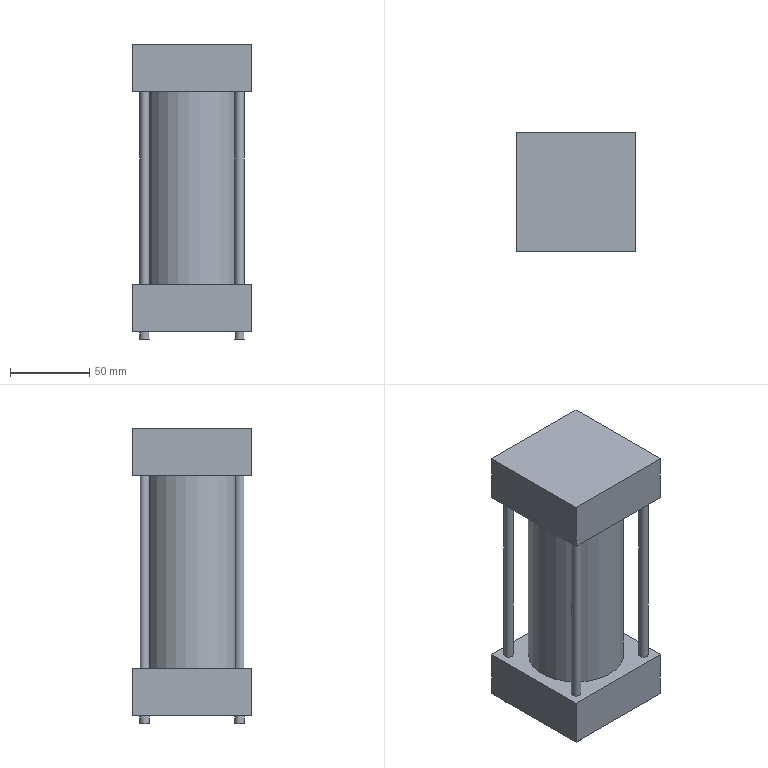Part | NX | features solid 2 | 1 solid | 29 faces | box 75 x 75 x 186 mm | volume 689867 mm3 | plane 16 | cylinder 13 | commonest cylinder face diameters 6 x8 60 x3 18 x2
STEP:
#1=CARTESIAN_POINT('',(168.,47.5,-150.));
#2=VERTEX_POINT('',#1);
#3=CARTESIAN_POINT('',(165.,47.5,-150.));
#4=DIRECTION('',(0.,0.,1.));
#5=DIRECTION('',(1.,0.,0.));
#6=AXIS2_PLACEMENT_3D('',#3,#4,#5);
#7=CIRCLE('',#6,3.);
#8=EDGE_CURVE('',#2,#2,#7,.F.);
#9=ORIENTED_EDGE('',*,*,#8,.F.);
#10=EDGE_LOOP('',(#9));
#11=FACE_BOUND('',#10,.T.);
#12=CARTESIAN_POINT('',(108.,47.5,-150.));
#13=VERTEX_POINT('',#12);
#14=CARTESIAN_POINT('',(105.,47.5,-150.));
#15=DIRECTION('',(0.,0.,1.));
#16=DIRECTION('',(1.,0.,0.));
#17=AXIS2_PLACEMENT_3D('',#14,#15,#16);
#18=CIRCLE('',#17,3.);
#19=EDGE_CURVE('',#13,#13,#18,.T.);
#20=ORIENTED_EDGE('',*,*,#19,.T.);
#21=EDGE_LOOP('',(#20));
#22=FACE_BOUND('',#21,.T.);
#23=CARTESIAN_POINT('',(97.5,115.,-150.));
#24=VERTEX_POINT('',#23);
#25=CARTESIAN_POINT('',(97.5,40.,-150.));
#26=VERTEX_POINT('',#25);
#27=CARTESIAN_POINT('',(97.5,112.5,-150.));
#28=DIRECTION('',(0.,-1.,0.));
#29=VECTOR('',#28,1000.);
#30=LINE('',#27,#29);
#31=EDGE_CURVE('',#24,#26,#30,.T.);
#32=ORIENTED_EDGE('',*,*,#31,.F.);
#33=CARTESIAN_POINT('',(172.5,115.,-150.));
#34=VERTEX_POINT('',#33);
#35=CARTESIAN_POINT('',(170.,115.,-150.));
#36=DIRECTION('',(-1.,0.,0.));
#37=VECTOR('',#36,1000.);
#38=LINE('',#35,#37);
#39=EDGE_CURVE('',#34,#24,#38,.T.);
#40=ORIENTED_EDGE('',*,*,#39,.F.);
#41=CARTESIAN_POINT('',(172.5,40.,-150.));
#42=VERTEX_POINT('',#41);
#43=CARTESIAN_POINT('',(172.5,42.5,-150.));
#44=DIRECTION('',(0.,1.,0.));
#45=VECTOR('',#44,1000.);
#46=LINE('',#43,#45);
#47=EDGE_CURVE('',#42,#34,#46,.T.);
#48=ORIENTED_EDGE('',*,*,#47,.F.);
#49=CARTESIAN_POINT('',(100.,40.,-150.));
#50=DIRECTION('',(1.,0.,0.));
#51=VECTOR('',#50,1000.);
#52=LINE('',#49,#51);
#53=EDGE_CURVE('',#26,#42,#52,.T.);
#54=ORIENTED_EDGE('',*,*,#53,.F.);
#55=EDGE_LOOP('',(#32,#40,#48,#54));
#56=FACE_BOUND('',#55,.T.);
#57=CARTESIAN_POINT('',(168.,107.5,-150.));
#58=VERTEX_POINT('',#57);
#59=CARTESIAN_POINT('',(165.,107.5,-150.));
#60=DIRECTION('',(0.,0.,1.));
#61=DIRECTION('',(1.,0.,0.));
#62=AXIS2_PLACEMENT_3D('',#59,#60,#61);
#63=CIRCLE('',#62,3.);
#64=EDGE_CURVE('',#58,#58,#63,.T.);
#65=ORIENTED_EDGE('',*,*,#64,.T.);
#66=EDGE_LOOP('',(#65));
#67=FACE_BOUND('',#66,.T.);
#68=CARTESIAN_POINT('',(108.,107.5,-150.));
#69=VERTEX_POINT('',#68);
#70=CARTESIAN_POINT('',(105.,107.5,-150.));
#71=DIRECTION('',(0.,0.,1.));
#72=DIRECTION('',(1.,0.,0.));
#73=AXIS2_PLACEMENT_3D('',#70,#71,#72);
#74=CIRCLE('',#73,3.);
#75=EDGE_CURVE('',#69,#69,#74,.F.);
#76=ORIENTED_EDGE('',*,*,#75,.F.);
#77=EDGE_LOOP('',(#76));
#78=FACE_BOUND('',#77,.T.);
#79=CARTESIAN_POINT('',(165.,77.5,-150.));
#80=VERTEX_POINT('',#79);
#81=CARTESIAN_POINT('',(135.,77.5,-150.));
#82=DIRECTION('',(0.,0.,1.));
#83=DIRECTION('',(1.,0.,0.));
#84=AXIS2_PLACEMENT_3D('',#81,#82,#83);
#85=CIRCLE('',#84,30.);
#86=EDGE_CURVE('',#80,#80,#85,.F.);
#87=ORIENTED_EDGE('',*,*,#86,.F.);
#88=EDGE_LOOP('',(#87));
#89=FACE_BOUND('',#88,.T.);
#90=CARTESIAN_POINT('',(100.,42.5,-150.));
#91=DIRECTION('',(0.,0.,-1.));
#92=DIRECTION('',(1.,0.,0.));
#93=AXIS2_PLACEMENT_3D('',#90,#91,#92);
#94=PLANE('',#93);
#95=ADVANCED_FACE('',(#11,#22,#56,#67,#78,#89),#94,.T.);
#96=CARTESIAN_POINT('',(108.,107.5,-271.));
#97=VERTEX_POINT('',#96);
#98=CARTESIAN_POINT('',(105.,107.5,-271.));
#99=DIRECTION('',(0.,0.,1.));
#100=DIRECTION('',(1.,0.,0.));
#101=AXIS2_PLACEMENT_3D('',#98,#99,#100);
#102=CIRCLE('',#101,3.);
#103=EDGE_CURVE('',#97,#97,#102,.T.);
#104=ORIENTED_EDGE('',*,*,#103,.F.);
#105=EDGE_LOOP('',(#104));
#106=FACE_BOUND('',#105,.T.);
#107=CARTESIAN_POINT('',(108.,47.5,-271.));
#108=VERTEX_POINT('',#107);
#109=CARTESIAN_POINT('',(105.,47.5,-271.));
#110=DIRECTION('',(0.,0.,1.));
#111=DIRECTION('',(1.,0.,0.));
#112=AXIS2_PLACEMENT_3D('',#109,#110,#111);
#113=CIRCLE('',#112,3.);
#114=EDGE_CURVE('',#108,#108,#113,.F.);
#115=ORIENTED_EDGE('',*,*,#114,.T.);
#116=EDGE_LOOP('',(#115));
#117=FACE_BOUND('',#116,.T.);
#118=CARTESIAN_POINT('',(172.5,40.,-271.));
#119=VERTEX_POINT('',#118);
#120=CARTESIAN_POINT('',(172.5,115.,-271.));
#121=VERTEX_POINT('',#120);
#122=CARTESIAN_POINT('',(172.5,42.5,-271.));
#123=DIRECTION('',(0.,1.,0.));
#124=VECTOR('',#123,1000.);
#125=LINE('',#122,#124);
#126=EDGE_CURVE('',#119,#121,#125,.T.);
#127=ORIENTED_EDGE('',*,*,#126,.T.);
#128=CARTESIAN_POINT('',(97.5,115.,-271.));
#129=VERTEX_POINT('',#128);
#130=CARTESIAN_POINT('',(170.,115.,-271.));
#131=DIRECTION('',(-1.,0.,0.));
#132=VECTOR('',#131,1000.);
#133=LINE('',#130,#132);
#134=EDGE_CURVE('',#121,#129,#133,.T.);
#135=ORIENTED_EDGE('',*,*,#134,.T.);
#136=CARTESIAN_POINT('',(97.5,40.,-271.));
#137=VERTEX_POINT('',#136);
#138=CARTESIAN_POINT('',(97.5,112.5,-271.));
#139=DIRECTION('',(0.,-1.,0.));
#140=VECTOR('',#139,1000.);
#141=LINE('',#138,#140);
#142=EDGE_CURVE('',#129,#137,#141,.T.);
#143=ORIENTED_EDGE('',*,*,#142,.T.);
#144=CARTESIAN_POINT('',(100.,40.,-271.));
#145=DIRECTION('',(1.,0.,0.));
#146=VECTOR('',#145,1000.);
#147=LINE('',#144,#146);
#148=EDGE_CURVE('',#137,#119,#147,.T.);
#149=ORIENTED_EDGE('',*,*,#148,.T.);
#150=EDGE_LOOP('',(#127,#135,#143,#149));
#151=FACE_BOUND('',#150,.T.);
#152=CARTESIAN_POINT('',(168.,47.5,-271.));
#153=VERTEX_POINT('',#152);
#154=CARTESIAN_POINT('',(165.,47.5,-271.));
#155=DIRECTION('',(0.,0.,1.));
#156=DIRECTION('',(1.,0.,0.));
#157=AXIS2_PLACEMENT_3D('',#154,#155,#156);
#158=CIRCLE('',#157,3.);
#159=EDGE_CURVE('',#153,#153,#158,.T.);
#160=ORIENTED_EDGE('',*,*,#159,.F.);
#161=EDGE_LOOP('',(#160));
#162=FACE_BOUND('',#161,.T.);
#163=CARTESIAN_POINT('',(168.,107.5,-271.));
#164=VERTEX_POINT('',#163);
#165=CARTESIAN_POINT('',(165.,107.5,-271.));
#166=DIRECTION('',(0.,0.,1.));
#167=DIRECTION('',(1.,0.,0.));
#168=AXIS2_PLACEMENT_3D('',#165,#166,#167);
#169=CIRCLE('',#168,3.);
#170=EDGE_CURVE('',#164,#164,#169,.F.);
#171=ORIENTED_EDGE('',*,*,#170,.T.);
#172=EDGE_LOOP('',(#171));
#173=FACE_BOUND('',#172,.T.);
#174=CARTESIAN_POINT('',(165.,77.5,-271.));
#175=VERTEX_POINT('',#174);
#176=CARTESIAN_POINT('',(135.,77.5,-271.));
#177=DIRECTION('',(0.,0.,1.));
#178=DIRECTION('',(1.,0.,0.));
#179=AXIS2_PLACEMENT_3D('',#176,#177,#178);
#180=CIRCLE('',#179,30.);
#181=EDGE_CURVE('',#175,#175,#180,.F.);
#182=ORIENTED_EDGE('',*,*,#181,.T.);
#183=EDGE_LOOP('',(#182));
#184=FACE_BOUND('',#183,.T.);
#185=CARTESIAN_POINT('',(170.,112.5,-271.));
#186=DIRECTION('',(0.,0.,-1.));
#187=DIRECTION('',(1.,0.,0.));
#188=AXIS2_PLACEMENT_3D('',#185,#186,#187);
#189=PLANE('',#188);
#190=ADVANCED_FACE('',(#106,#117,#151,#162,#173,#184),#189,.F.);
#191=CARTESIAN_POINT('',(134.391,115.,-144.));
#192=VERTEX_POINT('',#191);
#193=CARTESIAN_POINT('',(134.391,115.,-135.));
#194=DIRECTION('',(0.,1.,0.));
#195=DIRECTION('',(0.,0.,-1.));
#196=AXIS2_PLACEMENT_3D('',#193,#194,#195);
#197=CIRCLE('',#196,9.);
#198=EDGE_CURVE('',#192,#192,#197,.T.);
#199=ORIENTED_EDGE('',*,*,#198,.T.);
#200=EDGE_LOOP('',(#199));
#201=FACE_BOUND('',#200,.T.);
#202=CARTESIAN_POINT('',(134.391,107.494,-144.));
#203=VERTEX_POINT('',#202);
#204=CARTESIAN_POINT('',(127.349,106.676,-142.056));
#205=CARTESIAN_POINT('',(134.384,107.832,-144.976));
#206=CARTESIAN_POINT('',(141.46,106.961,-142.04));
#207=CARTESIAN_POINT('',(144.365,105.971,-134.989));
#208=CARTESIAN_POINT('',(141.426,106.97,-127.921));
#209=CARTESIAN_POINT('',(134.345,107.83,-125.028));
#210=CARTESIAN_POINT('',(127.326,106.668,-127.966));
#211=CARTESIAN_POINT('',(124.418,105.543,-135.02));
#212=CARTESIAN_POINT('',(127.349,106.676,-142.056));
#213=CARTESIAN_POINT('',(134.384,107.832,-144.976));
#214=CARTESIAN_POINT('',(141.46,106.961,-142.04));
#215=B_SPLINE_CURVE_WITH_KNOTS('',3,(#204,#205,#206,#207,#208,#209,#210,#211,#212,#213,#214),.UNSPECIFIED.,.T.,.F.,(1,1,1,1,1,1,1,1,1,1,1,1,1,1,1),(-0.02123,-0.01415,-0.007076,0.,0.007076,0.01415,0.02123,0.0283,0.03538,0.04245,0.04953,0.05661,0.06368,0.07076,0.07783),.UNSPECIFIED.);
#216=EDGE_CURVE('',#203,#203,#215,.T.);
#217=ORIENTED_EDGE('',*,*,#216,.T.);
#218=EDGE_LOOP('',(#217));
#219=FACE_BOUND('',#218,.T.);
#220=CARTESIAN_POINT('',(134.391,112.5,-135.));
#221=DIRECTION('',(0.,-1.,0.));
#222=DIRECTION('',(0.,0.,-1.));
#223=AXIS2_PLACEMENT_3D('',#220,#221,#222);
#224=CYLINDRICAL_SURFACE('',#223,9.);
#225=ADVANCED_FACE('',(#201,#219),#224,.F.);
#226=CARTESIAN_POINT('',(136.023,115.,-295.));
#227=VERTEX_POINT('',#226);
#228=CARTESIAN_POINT('',(136.023,115.,-286.));
#229=DIRECTION('',(0.,1.,0.));
#230=DIRECTION('',(0.,0.,-1.));
#231=AXIS2_PLACEMENT_3D('',#228,#229,#230);
#232=CIRCLE('',#231,9.);
#233=EDGE_CURVE('',#227,#227,#232,.T.);
#234=ORIENTED_EDGE('',*,*,#233,.T.);
#235=EDGE_LOOP('',(#234));
#236=FACE_BOUND('',#235,.T.);
#237=CARTESIAN_POINT('',(136.023,107.483,-295.));
#238=VERTEX_POINT('',#237);
#239=CARTESIAN_POINT('',(128.942,107.046,-293.036));
#240=CARTESIAN_POINT('',(136.036,107.82,-295.976));
#241=CARTESIAN_POINT('',(143.052,106.569,-293.06));
#242=CARTESIAN_POINT('',(145.997,105.384,-286.05));
#243=CARTESIAN_POINT('',(143.099,106.552,-278.981));
#244=CARTESIAN_POINT('',(136.115,107.817,-276.03));
#245=CARTESIAN_POINT('',(129.003,107.061,-278.902));
#246=CARTESIAN_POINT('',(126.049,106.104,-285.962));
#247=CARTESIAN_POINT('',(128.942,107.046,-293.036));
#248=CARTESIAN_POINT('',(136.036,107.82,-295.976));
#249=CARTESIAN_POINT('',(143.052,106.569,-293.06));
#250=B_SPLINE_CURVE_WITH_KNOTS('',3,(#239,#240,#241,#242,#243,#244,#245,#246,#247,#248,#249),.UNSPECIFIED.,.T.,.F.,(1,1,1,1,1,1,1,1,1,1,1,1,1,1,1),(-0.02123,-0.01415,-0.007076,0.,0.007076,0.01415,0.02123,0.0283,0.03538,0.04246,0.04953,0.05661,0.06368,0.07076,0.07784),.UNSPECIFIED.);
#251=EDGE_CURVE('',#238,#238,#250,.T.);
#252=ORIENTED_EDGE('',*,*,#251,.T.);
#253=EDGE_LOOP('',(#252));
#254=FACE_BOUND('',#253,.T.);
#255=CARTESIAN_POINT('',(136.023,112.5,-286.));
#256=DIRECTION('',(0.,-1.,0.));
#257=DIRECTION('',(0.,0.,-1.));
#258=AXIS2_PLACEMENT_3D('',#255,#256,#257);
#259=CYLINDRICAL_SURFACE('',#258,9.);
#260=ADVANCED_FACE('',(#236,#254),#259,.F.);
#261=ORIENTED_EDGE('',*,*,#64,.F.);
#262=EDGE_LOOP('',(#261));
#263=FACE_BOUND('',#262,.T.);
#264=ORIENTED_EDGE('',*,*,#170,.F.);
#265=EDGE_LOOP('',(#264));
#266=FACE_BOUND('',#265,.T.);
#267=CARTESIAN_POINT('',(165.,107.5,-306.));
#268=DIRECTION('',(0.,0.,1.));
#269=DIRECTION('',(-1.,0.,0.));
#270=AXIS2_PLACEMENT_3D('',#267,#268,#269);
#271=CYLINDRICAL_SURFACE('',#270,3.);
#272=ADVANCED_FACE('',(#263,#266),#271,.T.);
#273=ORIENTED_EDGE('',*,*,#75,.T.);
#274=EDGE_LOOP('',(#273));
#275=FACE_BOUND('',#274,.T.);
#276=ORIENTED_EDGE('',*,*,#103,.T.);
#277=EDGE_LOOP('',(#276));
#278=FACE_BOUND('',#277,.T.);
#279=CARTESIAN_POINT('',(105.,107.5,-306.));
#280=DIRECTION('',(0.,0.,1.));
#281=DIRECTION('',(-1.,0.,0.));
#282=AXIS2_PLACEMENT_3D('',#279,#280,#281);
#283=CYLINDRICAL_SURFACE('',#282,3.);
#284=ADVANCED_FACE('',(#275,#278),#283,.T.);
#285=ORIENTED_EDGE('',*,*,#19,.F.);
#286=EDGE_LOOP('',(#285));
#287=FACE_BOUND('',#286,.T.);
#288=ORIENTED_EDGE('',*,*,#114,.F.);
#289=EDGE_LOOP('',(#288));
#290=FACE_BOUND('',#289,.T.);
#291=CARTESIAN_POINT('',(105.,47.5,-306.));
#292=DIRECTION('',(0.,0.,1.));
#293=DIRECTION('',(-1.,0.,0.));
#294=AXIS2_PLACEMENT_3D('',#291,#292,#293);
#295=CYLINDRICAL_SURFACE('',#294,3.);
#296=ADVANCED_FACE('',(#287,#290),#295,.T.);
#297=ORIENTED_EDGE('',*,*,#8,.T.);
#298=EDGE_LOOP('',(#297));
#299=FACE_BOUND('',#298,.T.);
#300=ORIENTED_EDGE('',*,*,#159,.T.);
#301=EDGE_LOOP('',(#300));
#302=FACE_BOUND('',#301,.T.);
#303=CARTESIAN_POINT('',(165.,47.5,-306.));
#304=DIRECTION('',(0.,0.,1.));
#305=DIRECTION('',(-1.,0.,0.));
#306=AXIS2_PLACEMENT_3D('',#303,#304,#305);
#307=CYLINDRICAL_SURFACE('',#306,3.);
#308=ADVANCED_FACE('',(#299,#302),#307,.T.);
#309=CARTESIAN_POINT('',(97.5,115.,-120.));
#310=VERTEX_POINT('',#309);
#311=CARTESIAN_POINT('',(97.5,40.,-120.));
#312=VERTEX_POINT('',#311);
#313=CARTESIAN_POINT('',(97.5,112.5,-120.));
#314=DIRECTION('',(0.,-1.,0.));
#315=VECTOR('',#314,1000.);
#316=LINE('',#313,#315);
#317=EDGE_CURVE('',#310,#312,#316,.T.);
#318=ORIENTED_EDGE('',*,*,#317,.F.);
#319=CARTESIAN_POINT('',(97.5,115.,-150.));
#320=DIRECTION('',(0.,0.,1.));
#321=VECTOR('',#320,1000.);
#322=LINE('',#319,#321);
#323=EDGE_CURVE('',#24,#310,#322,.T.);
#324=ORIENTED_EDGE('',*,*,#323,.F.);
#325=ORIENTED_EDGE('',*,*,#31,.T.);
#326=CARTESIAN_POINT('',(97.5,40.,-150.));
#327=DIRECTION('',(0.,0.,1.));
#328=VECTOR('',#327,1000.);
#329=LINE('',#326,#328);
#330=EDGE_CURVE('',#26,#312,#329,.T.);
#331=ORIENTED_EDGE('',*,*,#330,.T.);
#332=EDGE_LOOP('',(#318,#324,#325,#331));
#333=FACE_BOUND('',#332,.T.);
#334=CARTESIAN_POINT('',(97.5,112.5,-150.));
#335=DIRECTION('',(1.,0.,0.));
#336=DIRECTION('',(0.,-1.,0.));
#337=AXIS2_PLACEMENT_3D('',#334,#335,#336);
#338=PLANE('',#337);
#339=ADVANCED_FACE('',(#333),#338,.F.);
#340=CARTESIAN_POINT('',(172.5,40.,-120.));
#341=VERTEX_POINT('',#340);
#342=CARTESIAN_POINT('',(100.,40.,-120.));
#343=DIRECTION('',(1.,0.,0.));
#344=VECTOR('',#343,1000.);
#345=LINE('',#342,#344);
#346=EDGE_CURVE('',#312,#341,#345,.T.);
#347=ORIENTED_EDGE('',*,*,#346,.F.);
#348=ORIENTED_EDGE('',*,*,#330,.F.);
#349=ORIENTED_EDGE('',*,*,#53,.T.);
#350=CARTESIAN_POINT('',(172.5,40.,-150.));
#351=DIRECTION('',(0.,0.,1.));
#352=VECTOR('',#351,1000.);
#353=LINE('',#350,#352);
#354=EDGE_CURVE('',#42,#341,#353,.T.);
#355=ORIENTED_EDGE('',*,*,#354,.T.);
#356=EDGE_LOOP('',(#347,#348,#349,#355));
#357=FACE_BOUND('',#356,.T.);
#358=CARTESIAN_POINT('',(100.,40.,-150.));
#359=DIRECTION('',(0.,1.,0.));
#360=DIRECTION('',(1.,0.,0.));
#361=AXIS2_PLACEMENT_3D('',#358,#359,#360);
#362=PLANE('',#361);
#363=ADVANCED_FACE('',(#357),#362,.F.);
#364=CARTESIAN_POINT('',(172.5,115.,-120.));
#365=VERTEX_POINT('',#364);
#366=CARTESIAN_POINT('',(172.5,42.5,-120.));
#367=DIRECTION('',(0.,1.,0.));
#368=VECTOR('',#367,1000.);
#369=LINE('',#366,#368);
#370=EDGE_CURVE('',#341,#365,#369,.T.);
#371=ORIENTED_EDGE('',*,*,#370,.F.);
#372=ORIENTED_EDGE('',*,*,#354,.F.);
#373=ORIENTED_EDGE('',*,*,#47,.T.);
#374=CARTESIAN_POINT('',(172.5,115.,-150.));
#375=DIRECTION('',(0.,0.,1.));
#376=VECTOR('',#375,1000.);
#377=LINE('',#374,#376);
#378=EDGE_CURVE('',#34,#365,#377,.T.);
#379=ORIENTED_EDGE('',*,*,#378,.T.);
#380=EDGE_LOOP('',(#371,#372,#373,#379));
#381=FACE_BOUND('',#380,.T.);
#382=CARTESIAN_POINT('',(172.5,42.5,-150.));
#383=DIRECTION('',(-1.,0.,0.));
#384=DIRECTION('',(0.,0.,-1.));
#385=AXIS2_PLACEMENT_3D('',#382,#383,#384);
#386=PLANE('',#385);
#387=ADVANCED_FACE('',(#381),#386,.F.);
#388=ORIENTED_EDGE('',*,*,#198,.F.);
#389=EDGE_LOOP('',(#388));
#390=FACE_BOUND('',#389,.T.);
#391=CARTESIAN_POINT('',(170.,115.,-120.));
#392=DIRECTION('',(-1.,0.,0.));
#393=VECTOR('',#392,1000.);
#394=LINE('',#391,#393);
#395=EDGE_CURVE('',#365,#310,#394,.T.);
#396=ORIENTED_EDGE('',*,*,#395,.F.);
#397=ORIENTED_EDGE('',*,*,#378,.F.);
#398=ORIENTED_EDGE('',*,*,#39,.T.);
#399=ORIENTED_EDGE('',*,*,#323,.T.);
#400=EDGE_LOOP('',(#396,#397,#398,#399));
#401=FACE_BOUND('',#400,.T.);
#402=CARTESIAN_POINT('',(170.,115.,-150.));
#403=DIRECTION('',(0.,-1.,0.));
#404=DIRECTION('',(0.,0.,-1.));
#405=AXIS2_PLACEMENT_3D('',#402,#403,#404);
#406=PLANE('',#405);
#407=ADVANCED_FACE('',(#390,#401),#406,.F.);
#408=ORIENTED_EDGE('',*,*,#317,.T.);
#409=ORIENTED_EDGE('',*,*,#346,.T.);
#410=ORIENTED_EDGE('',*,*,#370,.T.);
#411=ORIENTED_EDGE('',*,*,#395,.T.);
#412=EDGE_LOOP('',(#408,#409,#410,#411));
#413=FACE_BOUND('',#412,.T.);
#414=CARTESIAN_POINT('',(100.,42.5,-120.));
#415=DIRECTION('',(0.,0.,-1.));
#416=DIRECTION('',(1.,0.,0.));
#417=AXIS2_PLACEMENT_3D('',#414,#415,#416);
#418=PLANE('',#417);
#419=ADVANCED_FACE('',(#413),#418,.F.);
#420=CARTESIAN_POINT('',(168.,107.5,-301.));
#421=VERTEX_POINT('',#420);
#422=CARTESIAN_POINT('',(165.,107.5,-301.));
#423=DIRECTION('',(0.,0.,1.));
#424=DIRECTION('',(1.,0.,0.));
#425=AXIS2_PLACEMENT_3D('',#422,#423,#424);
#426=CIRCLE('',#425,3.);
#427=EDGE_CURVE('',#421,#421,#426,.F.);
#428=ORIENTED_EDGE('',*,*,#427,.F.);
#429=EDGE_LOOP('',(#428));
#430=FACE_BOUND('',#429,.T.);
#431=CARTESIAN_POINT('',(168.,47.5,-301.));
#432=VERTEX_POINT('',#431);
#433=CARTESIAN_POINT('',(165.,47.5,-301.));
#434=DIRECTION('',(0.,0.,1.));
#435=DIRECTION('',(1.,0.,0.));
#436=AXIS2_PLACEMENT_3D('',#433,#434,#435);
#437=CIRCLE('',#436,3.);
#438=EDGE_CURVE('',#432,#432,#437,.T.);
#439=ORIENTED_EDGE('',*,*,#438,.T.);
#440=EDGE_LOOP('',(#439));
#441=FACE_BOUND('',#440,.T.);
#442=CARTESIAN_POINT('',(172.5,40.,-301.));
#443=VERTEX_POINT('',#442);
#444=CARTESIAN_POINT('',(172.5,115.,-301.));
#445=VERTEX_POINT('',#444);
#446=CARTESIAN_POINT('',(172.5,42.5,-301.));
#447=DIRECTION('',(0.,1.,0.));
#448=VECTOR('',#447,1000.);
#449=LINE('',#446,#448);
#450=EDGE_CURVE('',#443,#445,#449,.T.);
#451=ORIENTED_EDGE('',*,*,#450,.F.);
#452=CARTESIAN_POINT('',(97.5,40.,-301.));
#453=VERTEX_POINT('',#452);
#454=CARTESIAN_POINT('',(100.,40.,-301.));
#455=DIRECTION('',(1.,0.,0.));
#456=VECTOR('',#455,1000.);
#457=LINE('',#454,#456);
#458=EDGE_CURVE('',#453,#443,#457,.T.);
#459=ORIENTED_EDGE('',*,*,#458,.F.);
#460=CARTESIAN_POINT('',(97.5,115.,-301.));
#461=VERTEX_POINT('',#460);
#462=CARTESIAN_POINT('',(97.5,112.5,-301.));
#463=DIRECTION('',(0.,-1.,0.));
#464=VECTOR('',#463,1000.);
#465=LINE('',#462,#464);
#466=EDGE_CURVE('',#461,#453,#465,.T.);
#467=ORIENTED_EDGE('',*,*,#466,.F.);
#468=CARTESIAN_POINT('',(170.,115.,-301.));
#469=DIRECTION('',(-1.,0.,0.));
#470=VECTOR('',#469,1000.);
#471=LINE('',#468,#470);
#472=EDGE_CURVE('',#445,#461,#471,.T.);
#473=ORIENTED_EDGE('',*,*,#472,.F.);
#474=EDGE_LOOP('',(#451,#459,#467,#473));
#475=FACE_BOUND('',#474,.T.);
#476=CARTESIAN_POINT('',(108.,47.5,-301.));
#477=VERTEX_POINT('',#476);
#478=CARTESIAN_POINT('',(105.,47.5,-301.));
#479=DIRECTION('',(0.,0.,1.));
#480=DIRECTION('',(1.,0.,0.));
#481=AXIS2_PLACEMENT_3D('',#478,#479,#480);
#482=CIRCLE('',#481,3.);
#483=EDGE_CURVE('',#477,#477,#482,.F.);
#484=ORIENTED_EDGE('',*,*,#483,.F.);
#485=EDGE_LOOP('',(#484));
#486=FACE_BOUND('',#485,.T.);
#487=CARTESIAN_POINT('',(108.,107.5,-301.));
#488=VERTEX_POINT('',#487);
#489=CARTESIAN_POINT('',(105.,107.5,-301.));
#490=DIRECTION('',(0.,0.,1.));
#491=DIRECTION('',(1.,0.,0.));
#492=AXIS2_PLACEMENT_3D('',#489,#490,#491);
#493=CIRCLE('',#492,3.);
#494=EDGE_CURVE('',#488,#488,#493,.T.);
#495=ORIENTED_EDGE('',*,*,#494,.T.);
#496=EDGE_LOOP('',(#495));
#497=FACE_BOUND('',#496,.T.);
#498=CARTESIAN_POINT('',(170.,112.5,-301.));
#499=DIRECTION('',(0.,0.,-1.));
#500=DIRECTION('',(1.,0.,0.));
#501=AXIS2_PLACEMENT_3D('',#498,#499,#500);
#502=PLANE('',#501);
#503=ADVANCED_FACE('',(#430,#441,#475,#486,#497),#502,.T.);
#504=ORIENTED_EDGE('',*,*,#126,.F.);
#505=CARTESIAN_POINT('',(172.5,40.,-301.));
#506=DIRECTION('',(0.,0.,1.));
#507=VECTOR('',#506,1000.);
#508=LINE('',#505,#507);
#509=EDGE_CURVE('',#443,#119,#508,.T.);
#510=ORIENTED_EDGE('',*,*,#509,.F.);
#511=ORIENTED_EDGE('',*,*,#450,.T.);
#512=CARTESIAN_POINT('',(172.5,115.,-301.));
#513=DIRECTION('',(0.,0.,1.));
#514=VECTOR('',#513,1000.);
#515=LINE('',#512,#514);
#516=EDGE_CURVE('',#445,#121,#515,.T.);
#517=ORIENTED_EDGE('',*,*,#516,.T.);
#518=EDGE_LOOP('',(#504,#510,#511,#517));
#519=FACE_BOUND('',#518,.T.);
#520=CARTESIAN_POINT('',(172.5,42.5,-301.));
#521=DIRECTION('',(-1.,0.,0.));
#522=DIRECTION('',(0.,0.,-1.));
#523=AXIS2_PLACEMENT_3D('',#520,#521,#522);
#524=PLANE('',#523);
#525=ADVANCED_FACE('',(#519),#524,.F.);
#526=ORIENTED_EDGE('',*,*,#233,.F.);
#527=EDGE_LOOP('',(#526));
#528=FACE_BOUND('',#527,.T.);
#529=ORIENTED_EDGE('',*,*,#134,.F.);
#530=ORIENTED_EDGE('',*,*,#516,.F.);
#531=ORIENTED_EDGE('',*,*,#472,.T.);
#532=CARTESIAN_POINT('',(97.5,115.,-301.));
#533=DIRECTION('',(0.,0.,1.));
#534=VECTOR('',#533,1000.);
#535=LINE('',#532,#534);
#536=EDGE_CURVE('',#461,#129,#535,.T.);
#537=ORIENTED_EDGE('',*,*,#536,.T.);
#538=EDGE_LOOP('',(#529,#530,#531,#537));
#539=FACE_BOUND('',#538,.T.);
#540=CARTESIAN_POINT('',(170.,115.,-301.));
#541=DIRECTION('',(0.,-1.,0.));
#542=DIRECTION('',(0.,0.,-1.));
#543=AXIS2_PLACEMENT_3D('',#540,#541,#542);
#544=PLANE('',#543);
#545=ADVANCED_FACE('',(#528,#539),#544,.F.);
#546=ORIENTED_EDGE('',*,*,#142,.F.);
#547=ORIENTED_EDGE('',*,*,#536,.F.);
#548=ORIENTED_EDGE('',*,*,#466,.T.);
#549=CARTESIAN_POINT('',(97.5,40.,-301.));
#550=DIRECTION('',(0.,0.,1.));
#551=VECTOR('',#550,1000.);
#552=LINE('',#549,#551);
#553=EDGE_CURVE('',#453,#137,#552,.T.);
#554=ORIENTED_EDGE('',*,*,#553,.T.);
#555=EDGE_LOOP('',(#546,#547,#548,#554));
#556=FACE_BOUND('',#555,.T.);
#557=CARTESIAN_POINT('',(97.5,112.5,-301.));
#558=DIRECTION('',(1.,0.,0.));
#559=DIRECTION('',(0.,-1.,0.));
#560=AXIS2_PLACEMENT_3D('',#557,#558,#559);
#561=PLANE('',#560);
#562=ADVANCED_FACE('',(#556),#561,.F.);
#563=ORIENTED_EDGE('',*,*,#148,.F.);
#564=ORIENTED_EDGE('',*,*,#553,.F.);
#565=ORIENTED_EDGE('',*,*,#458,.T.);
#566=ORIENTED_EDGE('',*,*,#509,.T.);
#567=EDGE_LOOP('',(#563,#564,#565,#566));
#568=FACE_BOUND('',#567,.T.);
#569=CARTESIAN_POINT('',(100.,40.,-301.));
#570=DIRECTION('',(0.,1.,0.));
#571=DIRECTION('',(1.,0.,0.));
#572=AXIS2_PLACEMENT_3D('',#569,#570,#571);
#573=PLANE('',#572);
#574=ADVANCED_FACE('',(#568),#573,.F.);
#575=CARTESIAN_POINT('',(165.,50.5,-306.));
#576=VERTEX_POINT('',#575);
#577=CARTESIAN_POINT('',(165.,47.5,-306.));
#578=DIRECTION('',(0.,0.,1.));
#579=DIRECTION('',(0.,1.,0.));
#580=AXIS2_PLACEMENT_3D('',#577,#578,#579);
#581=CIRCLE('',#580,3.);
#582=EDGE_CURVE('',#576,#576,#581,.T.);
#583=ORIENTED_EDGE('',*,*,#582,.F.);
#584=EDGE_LOOP('',(#583));
#585=FACE_BOUND('',#584,.T.);
#586=CARTESIAN_POINT('',(165.,47.5,-306.));
#587=DIRECTION('',(0.,0.,-1.));
#588=DIRECTION('',(1.,0.,0.));
#589=AXIS2_PLACEMENT_3D('',#586,#587,#588);
#590=PLANE('',#589);
#591=ADVANCED_FACE('',(#585),#590,.T.);
#592=ORIENTED_EDGE('',*,*,#438,.F.);
#593=EDGE_LOOP('',(#592));
#594=FACE_BOUND('',#593,.T.);
#595=ORIENTED_EDGE('',*,*,#582,.T.);
#596=EDGE_LOOP('',(#595));
#597=FACE_BOUND('',#596,.T.);
#598=CARTESIAN_POINT('',(165.,47.5,-306.));
#599=DIRECTION('',(0.,0.,1.));
#600=DIRECTION('',(-1.,0.,0.));
#601=AXIS2_PLACEMENT_3D('',#598,#599,#600);
#602=CYLINDRICAL_SURFACE('',#601,3.);
#603=ADVANCED_FACE('',(#594,#597),#602,.T.);
#604=CARTESIAN_POINT('',(105.,50.5,-306.));
#605=VERTEX_POINT('',#604);
#606=CARTESIAN_POINT('',(105.,47.5,-306.));
#607=DIRECTION('',(0.,0.,-1.));
#608=DIRECTION('',(0.,1.,0.));
#609=AXIS2_PLACEMENT_3D('',#606,#607,#608);
#610=CIRCLE('',#609,3.);
#611=EDGE_CURVE('',#605,#605,#610,.T.);
#612=ORIENTED_EDGE('',*,*,#611,.T.);
#613=EDGE_LOOP('',(#612));
#614=FACE_BOUND('',#613,.T.);
#615=CARTESIAN_POINT('',(105.,47.5,-306.));
#616=DIRECTION('',(0.,0.,1.));
#617=DIRECTION('',(-1.,0.,0.));
#618=AXIS2_PLACEMENT_3D('',#615,#616,#617);
#619=PLANE('',#618);
#620=ADVANCED_FACE('',(#614),#619,.F.);
#621=ORIENTED_EDGE('',*,*,#483,.T.);
#622=EDGE_LOOP('',(#621));
#623=FACE_BOUND('',#622,.T.);
#624=ORIENTED_EDGE('',*,*,#611,.F.);
#625=EDGE_LOOP('',(#624));
#626=FACE_BOUND('',#625,.T.);
#627=CARTESIAN_POINT('',(105.,47.5,-306.));
#628=DIRECTION('',(0.,0.,1.));
#629=DIRECTION('',(-1.,0.,0.));
#630=AXIS2_PLACEMENT_3D('',#627,#628,#629);
#631=CYLINDRICAL_SURFACE('',#630,3.);
#632=ADVANCED_FACE('',(#623,#626),#631,.T.);
#633=CARTESIAN_POINT('',(105.,104.5,-306.));
#634=VERTEX_POINT('',#633);
#635=CARTESIAN_POINT('',(105.,107.5,-306.));
#636=DIRECTION('',(0.,0.,1.));
#637=DIRECTION('',(0.,-1.,0.));
#638=AXIS2_PLACEMENT_3D('',#635,#636,#637);
#639=CIRCLE('',#638,3.);
#640=EDGE_CURVE('',#634,#634,#639,.T.);
#641=ORIENTED_EDGE('',*,*,#640,.F.);
#642=EDGE_LOOP('',(#641));
#643=FACE_BOUND('',#642,.T.);
#644=CARTESIAN_POINT('',(105.,107.5,-306.));
#645=DIRECTION('',(0.,0.,-1.));
#646=DIRECTION('',(1.,0.,0.));
#647=AXIS2_PLACEMENT_3D('',#644,#645,#646);
#648=PLANE('',#647);
#649=ADVANCED_FACE('',(#643),#648,.T.);
#650=ORIENTED_EDGE('',*,*,#494,.F.);
#651=EDGE_LOOP('',(#650));
#652=FACE_BOUND('',#651,.T.);
#653=ORIENTED_EDGE('',*,*,#640,.T.);
#654=EDGE_LOOP('',(#653));
#655=FACE_BOUND('',#654,.T.);
#656=CARTESIAN_POINT('',(105.,107.5,-306.));
#657=DIRECTION('',(0.,0.,1.));
#658=DIRECTION('',(-1.,0.,0.));
#659=AXIS2_PLACEMENT_3D('',#656,#657,#658);
#660=CYLINDRICAL_SURFACE('',#659,3.);
#661=ADVANCED_FACE('',(#652,#655),#660,.T.);
#662=CARTESIAN_POINT('',(165.,104.5,-306.));
#663=VERTEX_POINT('',#662);
#664=CARTESIAN_POINT('',(165.,107.5,-306.));
#665=DIRECTION('',(0.,0.,-1.));
#666=DIRECTION('',(0.,-1.,0.));
#667=AXIS2_PLACEMENT_3D('',#664,#665,#666);
#668=CIRCLE('',#667,3.);
#669=EDGE_CURVE('',#663,#663,#668,.T.);
#670=ORIENTED_EDGE('',*,*,#669,.T.);
#671=EDGE_LOOP('',(#670));
#672=FACE_BOUND('',#671,.T.);
#673=CARTESIAN_POINT('',(165.,107.5,-306.));
#674=DIRECTION('',(0.,0.,1.));
#675=DIRECTION('',(-1.,0.,0.));
#676=AXIS2_PLACEMENT_3D('',#673,#674,#675);
#677=PLANE('',#676);
#678=ADVANCED_FACE('',(#672),#677,.F.);
#679=ORIENTED_EDGE('',*,*,#427,.T.);
#680=EDGE_LOOP('',(#679));
#681=FACE_BOUND('',#680,.T.);
#682=ORIENTED_EDGE('',*,*,#669,.F.);
#683=EDGE_LOOP('',(#682));
#684=FACE_BOUND('',#683,.T.);
#685=CARTESIAN_POINT('',(165.,107.5,-306.));
#686=DIRECTION('',(0.,0.,1.));
#687=DIRECTION('',(-1.,0.,0.));
#688=AXIS2_PLACEMENT_3D('',#685,#686,#687);
#689=CYLINDRICAL_SURFACE('',#688,3.);
#690=ADVANCED_FACE('',(#681,#684),#689,.T.);
#691=ORIENTED_EDGE('',*,*,#251,.F.);
#692=EDGE_LOOP('',(#691));
#693=FACE_BOUND('',#692,.T.);
#694=CARTESIAN_POINT('',(135.,77.5,-296.));
#695=DIRECTION('',(0.,0.,1.));
#696=DIRECTION('',(-1.,0.,0.));
#697=AXIS2_PLACEMENT_3D('',#694,#695,#696);
#698=CYLINDRICAL_SURFACE('',#697,30.);
#699=ADVANCED_FACE('',(#693),#698,.T.);
#700=ORIENTED_EDGE('',*,*,#216,.F.);
#701=EDGE_LOOP('',(#700));
#702=FACE_BOUND('',#701,.T.);
#703=CARTESIAN_POINT('',(135.,77.5,-296.));
#704=DIRECTION('',(0.,0.,1.));
#705=DIRECTION('',(-1.,0.,0.));
#706=AXIS2_PLACEMENT_3D('',#703,#704,#705);
#707=CYLINDRICAL_SURFACE('',#706,30.);
#708=ADVANCED_FACE('',(#702),#707,.T.);
#709=ORIENTED_EDGE('',*,*,#86,.T.);
#710=EDGE_LOOP('',(#709));
#711=FACE_BOUND('',#710,.T.);
#712=ORIENTED_EDGE('',*,*,#181,.F.);
#713=EDGE_LOOP('',(#712));
#714=FACE_BOUND('',#713,.T.);
#715=CARTESIAN_POINT('',(135.,77.5,-296.));
#716=DIRECTION('',(0.,0.,1.));
#717=DIRECTION('',(-1.,0.,0.));
#718=AXIS2_PLACEMENT_3D('',#715,#716,#717);
#719=CYLINDRICAL_SURFACE('',#718,30.);
#720=ADVANCED_FACE('',(#711,#714),#719,.T.);
#721=CLOSED_SHELL('',(#95,#190,#225,#260,#272,#284,#296,#308,#339,#363,#387,#407,#419,#503,#525,#545,#562,#574,#591,#603,#620,#632,#649,#661,#678,#690,#699,#708,#720));
#722=MANIFOLD_SOLID_BREP('',#721);
#723=(LENGTH_UNIT()NAMED_UNIT(*)SI_UNIT(.MILLI.,.METRE.));
#724=UNCERTAINTY_MEASURE_WITH_UNIT(LENGTH_MEASURE(0.0508),#723,'','');
#725=(NAMED_UNIT(*)PLANE_ANGLE_UNIT()SI_UNIT($,.RADIAN.));
#726=(NAMED_UNIT(*)SI_UNIT($,.STERADIAN.)SOLID_ANGLE_UNIT());
#727=(GEOMETRIC_REPRESENTATION_CONTEXT(3)GLOBAL_UNCERTAINTY_ASSIGNED_CONTEXT((#724))GLOBAL_UNIT_ASSIGNED_CONTEXT((#723,#725,#726))REPRESENTATION_CONTEXT('',''));
#728=ADVANCED_BREP_SHAPE_REPRESENTATION('',(#722),#727);